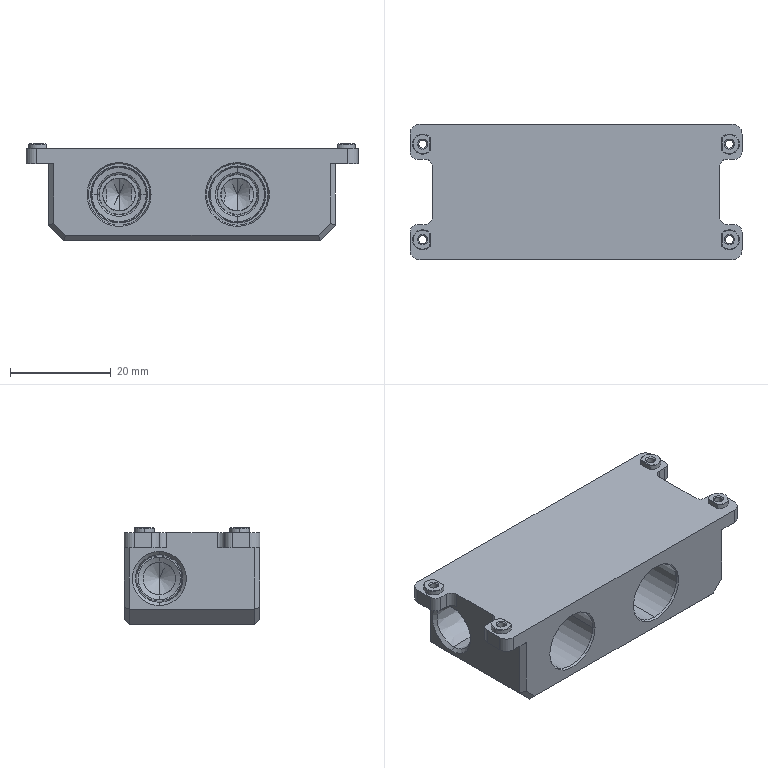Part | 1 solid | 157 faces | box 66 x 27 x 19.25 mm | volume 23061 mm3 | cylinder 56 | plane 47 | cone 42 | torus 12 | commonest cylinder face diameters 6.5 x16 4 x10 1.6 x8 3 x8 8.17 x4 11.15 x4